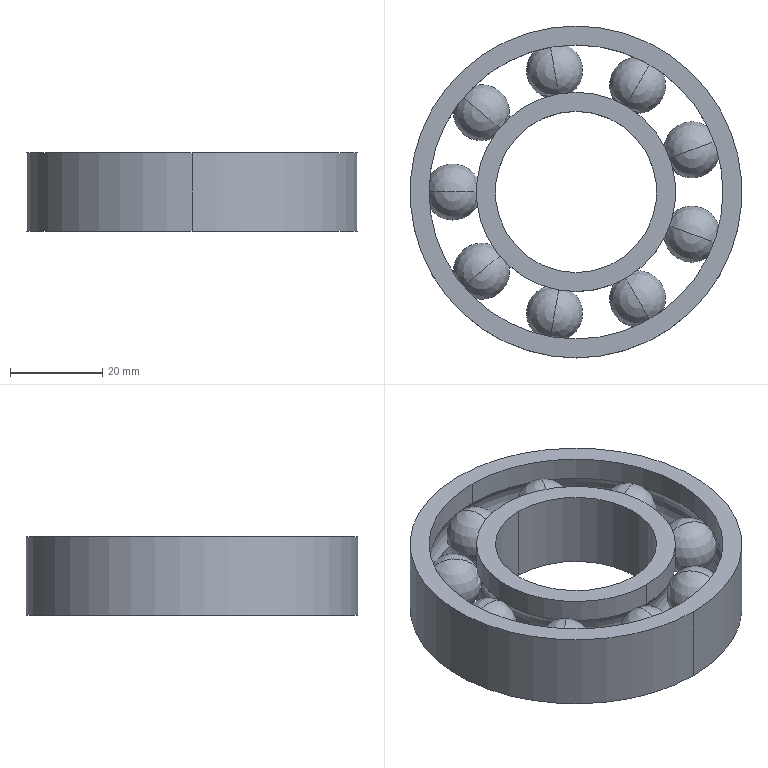Part | NX | features BREP 11 | 11 solids | 38 faces | box 72 x 72 x 17 mm | volume 30735 mm3 | sphere 18 | cylinder 12 | torus 4 | plane 4 | commonest cylinder face diameters 43.222 x4 63.778 x4 35 x2 72 x2
STEP:
#1=CARTESIAN_POINT('',(0.,21.611,3.409));
#2=VERTEX_POINT('',#1);
#3=CARTESIAN_POINT('',(0.,-21.611,3.409));
#4=VERTEX_POINT('',#3);
#5=CARTESIAN_POINT('',(0.,0.,3.409));
#6=DIRECTION('',(0.,0.,1.));
#7=DIRECTION('',(0.,1.,0.));
#8=AXIS2_PLACEMENT_3D('',#5,#6,#7);
#9=CIRCLE('',#8,21.611);
#10=EDGE_CURVE('',#2,#4,#9,.T.);
#11=ORIENTED_EDGE('',*,*,#10,.T.);
#12=CARTESIAN_POINT('',(0.,-21.611,8.5));
#13=VERTEX_POINT('',#12);
#14=CARTESIAN_POINT('',(0.,-21.611,3.409));
#15=DIRECTION('',(0.,0.,1.));
#16=VECTOR('',#15,1000.);
#17=LINE('',#14,#16);
#18=EDGE_CURVE('',#4,#13,#17,.T.);
#19=ORIENTED_EDGE('',*,*,#18,.T.);
#20=CARTESIAN_POINT('',(0.,21.611,8.5));
#21=VERTEX_POINT('',#20);
#22=CARTESIAN_POINT('',(0.,0.,8.5));
#23=DIRECTION('',(0.,0.,1.));
#24=DIRECTION('',(0.,1.,0.));
#25=AXIS2_PLACEMENT_3D('',#22,#23,#24);
#26=CIRCLE('',#25,21.611);
#27=EDGE_CURVE('',#21,#13,#26,.T.);
#28=ORIENTED_EDGE('',*,*,#27,.F.);
#29=CARTESIAN_POINT('',(0.,21.611,3.409));
#30=DIRECTION('',(0.,0.,1.));
#31=VECTOR('',#30,1000.);
#32=LINE('',#29,#31);
#33=EDGE_CURVE('',#2,#21,#32,.T.);
#34=ORIENTED_EDGE('',*,*,#33,.F.);
#35=EDGE_LOOP('',(#11,#19,#28,#34));
#36=FACE_BOUND('',#35,.T.);
#37=CARTESIAN_POINT('',(0.,0.,9.35));
#38=DIRECTION('',(0.,0.,-1.));
#39=DIRECTION('',(0.,1.,0.));
#40=AXIS2_PLACEMENT_3D('',#37,#38,#39);
#41=CYLINDRICAL_SURFACE('',#40,21.611);
#42=ADVANCED_FACE('',(#36),#41,.T.);
#43=CARTESIAN_POINT('',(0.,0.,8.5));
#44=DIRECTION('',(0.,0.,-1.));
#45=DIRECTION('',(0.,1.,0.));
#46=AXIS2_PLACEMENT_3D('',#43,#44,#45);
#47=CIRCLE('',#46,21.611);
#48=EDGE_CURVE('',#21,#13,#47,.T.);
#49=ORIENTED_EDGE('',*,*,#48,.T.);
#50=ORIENTED_EDGE('',*,*,#18,.F.);
#51=CARTESIAN_POINT('',(0.,0.,3.409));
#52=DIRECTION('',(0.,0.,-1.));
#53=DIRECTION('',(0.,1.,0.));
#54=AXIS2_PLACEMENT_3D('',#51,#52,#53);
#55=CIRCLE('',#54,21.611);
#56=EDGE_CURVE('',#2,#4,#55,.T.);
#57=ORIENTED_EDGE('',*,*,#56,.F.);
#58=ORIENTED_EDGE('',*,*,#33,.T.);
#59=EDGE_LOOP('',(#49,#50,#57,#58));
#60=FACE_BOUND('',#59,.T.);
#61=CARTESIAN_POINT('',(0.,0.,9.35));
#62=DIRECTION('',(0.,0.,-1.));
#63=DIRECTION('',(0.,1.,0.));
#64=AXIS2_PLACEMENT_3D('',#61,#62,#63);
#65=CYLINDRICAL_SURFACE('',#64,21.611);
#66=ADVANCED_FACE('',(#60),#65,.T.);
#67=ORIENTED_EDGE('',*,*,#56,.T.);
#68=CARTESIAN_POINT('',(0.,-21.611,-3.409));
#69=VERTEX_POINT('',#68);
#70=CARTESIAN_POINT('',(0.,-26.75,0.));
#71=DIRECTION('',(1.,0.,0.));
#72=DIRECTION('',(0.,0.8333,-0.5528));
#73=AXIS2_PLACEMENT_3D('',#70,#71,#72);
#74=CIRCLE('',#73,6.167);
#75=EDGE_CURVE('',#4,#69,#74,.F.);
#76=ORIENTED_EDGE('',*,*,#75,.T.);
#77=CARTESIAN_POINT('',(0.,21.611,-3.409));
#78=VERTEX_POINT('',#77);
#79=CARTESIAN_POINT('',(0.,0.,-3.409));
#80=DIRECTION('',(0.,0.,-1.));
#81=DIRECTION('',(0.,1.,0.));
#82=AXIS2_PLACEMENT_3D('',#79,#80,#81);
#83=CIRCLE('',#82,21.611);
#84=EDGE_CURVE('',#78,#69,#83,.T.);
#85=ORIENTED_EDGE('',*,*,#84,.F.);
#86=CARTESIAN_POINT('',(0.,26.75,0.));
#87=DIRECTION('',(-1.,0.,0.));
#88=DIRECTION('',(0.,-0.8333,-0.5528));
#89=AXIS2_PLACEMENT_3D('',#86,#87,#88);
#90=CIRCLE('',#89,6.167);
#91=EDGE_CURVE('',#2,#78,#90,.F.);
#92=ORIENTED_EDGE('',*,*,#91,.F.);
#93=EDGE_LOOP('',(#67,#76,#85,#92));
#94=FACE_BOUND('',#93,.T.);
#95=CARTESIAN_POINT('',(0.,0.,0.));
#96=DIRECTION('',(0.,0.,-1.));
#97=DIRECTION('',(0.,1.,0.));
#98=AXIS2_PLACEMENT_3D('',#95,#96,#97);
#99=TOROIDAL_SURFACE('',#98,26.75,6.167);
#100=ADVANCED_FACE('',(#94),#99,.F.);
#101=CARTESIAN_POINT('',(0.,0.,-3.409));
#102=DIRECTION('',(0.,0.,1.));
#103=DIRECTION('',(0.,1.,0.));
#104=AXIS2_PLACEMENT_3D('',#101,#102,#103);
#105=CIRCLE('',#104,21.611);
#106=EDGE_CURVE('',#78,#69,#105,.T.);
#107=ORIENTED_EDGE('',*,*,#106,.T.);
#108=ORIENTED_EDGE('',*,*,#75,.F.);
#109=ORIENTED_EDGE('',*,*,#10,.F.);
#110=ORIENTED_EDGE('',*,*,#91,.T.);
#111=EDGE_LOOP('',(#107,#108,#109,#110));
#112=FACE_BOUND('',#111,.T.);
#113=CARTESIAN_POINT('',(0.,0.,0.));
#114=DIRECTION('',(0.,0.,-1.));
#115=DIRECTION('',(0.,1.,0.));
#116=AXIS2_PLACEMENT_3D('',#113,#114,#115);
#117=TOROIDAL_SURFACE('',#116,26.75,6.167);
#118=ADVANCED_FACE('',(#112),#117,.F.);
#119=CARTESIAN_POINT('',(0.,21.611,-8.5));
#120=VERTEX_POINT('',#119);
#121=CARTESIAN_POINT('',(0.,-21.611,-8.5));
#122=VERTEX_POINT('',#121);
#123=CARTESIAN_POINT('',(0.,0.,-8.5));
#124=DIRECTION('',(0.,0.,1.));
#125=DIRECTION('',(0.,1.,0.));
#126=AXIS2_PLACEMENT_3D('',#123,#124,#125);
#127=CIRCLE('',#126,21.611);
#128=EDGE_CURVE('',#120,#122,#127,.T.);
#129=ORIENTED_EDGE('',*,*,#128,.T.);
#130=CARTESIAN_POINT('',(0.,-21.611,-8.5));
#131=DIRECTION('',(0.,0.,1.));
#132=VECTOR('',#131,1000.);
#133=LINE('',#130,#132);
#134=EDGE_CURVE('',#122,#69,#133,.T.);
#135=ORIENTED_EDGE('',*,*,#134,.T.);
#136=ORIENTED_EDGE('',*,*,#106,.F.);
#137=CARTESIAN_POINT('',(0.,21.611,-8.5));
#138=DIRECTION('',(0.,0.,1.));
#139=VECTOR('',#138,1000.);
#140=LINE('',#137,#139);
#141=EDGE_CURVE('',#120,#78,#140,.T.);
#142=ORIENTED_EDGE('',*,*,#141,.F.);
#143=EDGE_LOOP('',(#129,#135,#136,#142));
#144=FACE_BOUND('',#143,.T.);
#145=CARTESIAN_POINT('',(0.,0.,9.35));
#146=DIRECTION('',(0.,0.,-1.));
#147=DIRECTION('',(0.,1.,0.));
#148=AXIS2_PLACEMENT_3D('',#145,#146,#147);
#149=CYLINDRICAL_SURFACE('',#148,21.611);
#150=ADVANCED_FACE('',(#144),#149,.T.);
#151=ORIENTED_EDGE('',*,*,#84,.T.);
#152=ORIENTED_EDGE('',*,*,#134,.F.);
#153=CARTESIAN_POINT('',(0.,0.,-8.5));
#154=DIRECTION('',(0.,0.,-1.));
#155=DIRECTION('',(0.,1.,0.));
#156=AXIS2_PLACEMENT_3D('',#153,#154,#155);
#157=CIRCLE('',#156,21.611);
#158=EDGE_CURVE('',#120,#122,#157,.T.);
#159=ORIENTED_EDGE('',*,*,#158,.F.);
#160=ORIENTED_EDGE('',*,*,#141,.T.);
#161=EDGE_LOOP('',(#151,#152,#159,#160));
#162=FACE_BOUND('',#161,.T.);
#163=CARTESIAN_POINT('',(0.,0.,9.35));
#164=DIRECTION('',(0.,0.,-1.));
#165=DIRECTION('',(0.,1.,0.));
#166=AXIS2_PLACEMENT_3D('',#163,#164,#165);
#167=CYLINDRICAL_SURFACE('',#166,21.611);
#168=ADVANCED_FACE('',(#162),#167,.T.);
#169=ORIENTED_EDGE('',*,*,#128,.F.);
#170=ORIENTED_EDGE('',*,*,#158,.T.);
#171=EDGE_LOOP('',(#169,#170));
#172=FACE_BOUND('',#171,.T.);
#173=CARTESIAN_POINT('',(0.,17.5,-8.5));
#174=VERTEX_POINT('',#173);
#175=CARTESIAN_POINT('',(0.,-17.5,-8.5));
#176=VERTEX_POINT('',#175);
#177=CARTESIAN_POINT('',(0.,0.,-8.5));
#178=DIRECTION('',(0.,0.,-1.));
#179=DIRECTION('',(0.,1.,0.));
#180=AXIS2_PLACEMENT_3D('',#177,#178,#179);
#181=CIRCLE('',#180,17.5);
#182=EDGE_CURVE('',#174,#176,#181,.T.);
#183=ORIENTED_EDGE('',*,*,#182,.F.);
#184=CARTESIAN_POINT('',(0.,0.,-8.5));
#185=DIRECTION('',(0.,0.,1.));
#186=DIRECTION('',(0.,1.,0.));
#187=AXIS2_PLACEMENT_3D('',#184,#185,#186);
#188=CIRCLE('',#187,17.5);
#189=EDGE_CURVE('',#174,#176,#188,.T.);
#190=ORIENTED_EDGE('',*,*,#189,.T.);
#191=EDGE_LOOP('',(#183,#190));
#192=FACE_BOUND('',#191,.T.);
#193=CARTESIAN_POINT('',(0.,0.,-8.5));
#194=DIRECTION('',(0.,0.,-1.));
#195=DIRECTION('',(0.,1.,0.));
#196=AXIS2_PLACEMENT_3D('',#193,#194,#195);
#197=PLANE('',#196);
#198=ADVANCED_FACE('',(#172,#192),#197,.T.);
#199=CARTESIAN_POINT('',(0.,17.5,8.5));
#200=VERTEX_POINT('',#199);
#201=CARTESIAN_POINT('',(0.,-17.5,8.5));
#202=VERTEX_POINT('',#201);
#203=CARTESIAN_POINT('',(0.,0.,8.5));
#204=DIRECTION('',(0.,0.,1.));
#205=DIRECTION('',(0.,1.,0.));
#206=AXIS2_PLACEMENT_3D('',#203,#204,#205);
#207=CIRCLE('',#206,17.5);
#208=EDGE_CURVE('',#200,#202,#207,.T.);
#209=ORIENTED_EDGE('',*,*,#208,.T.);
#210=CARTESIAN_POINT('',(0.,-17.5,8.5));
#211=DIRECTION('',(0.,0.,-1.));
#212=VECTOR('',#211,1000.);
#213=LINE('',#210,#212);
#214=EDGE_CURVE('',#202,#176,#213,.T.);
#215=ORIENTED_EDGE('',*,*,#214,.T.);
#216=ORIENTED_EDGE('',*,*,#189,.F.);
#217=CARTESIAN_POINT('',(0.,17.5,8.5));
#218=DIRECTION('',(0.,0.,-1.));
#219=VECTOR('',#218,1000.);
#220=LINE('',#217,#219);
#221=EDGE_CURVE('',#200,#174,#220,.T.);
#222=ORIENTED_EDGE('',*,*,#221,.F.);
#223=EDGE_LOOP('',(#209,#215,#216,#222));
#224=FACE_BOUND('',#223,.T.);
#225=CARTESIAN_POINT('',(0.,0.,9.35));
#226=DIRECTION('',(0.,0.,-1.));
#227=DIRECTION('',(0.,1.,0.));
#228=AXIS2_PLACEMENT_3D('',#225,#226,#227);
#229=CYLINDRICAL_SURFACE('',#228,17.5);
#230=ADVANCED_FACE('',(#224),#229,.F.);
#231=ORIENTED_EDGE('',*,*,#182,.T.);
#232=ORIENTED_EDGE('',*,*,#214,.F.);
#233=CARTESIAN_POINT('',(0.,0.,8.5));
#234=DIRECTION('',(0.,0.,-1.));
#235=DIRECTION('',(0.,1.,0.));
#236=AXIS2_PLACEMENT_3D('',#233,#234,#235);
#237=CIRCLE('',#236,17.5);
#238=EDGE_CURVE('',#200,#202,#237,.T.);
#239=ORIENTED_EDGE('',*,*,#238,.F.);
#240=ORIENTED_EDGE('',*,*,#221,.T.);
#241=EDGE_LOOP('',(#231,#232,#239,#240));
#242=FACE_BOUND('',#241,.T.);
#243=CARTESIAN_POINT('',(0.,0.,9.35));
#244=DIRECTION('',(0.,0.,-1.));
#245=DIRECTION('',(0.,1.,0.));
#246=AXIS2_PLACEMENT_3D('',#243,#244,#245);
#247=CYLINDRICAL_SURFACE('',#246,17.5);
#248=ADVANCED_FACE('',(#242),#247,.F.);
#249=ORIENTED_EDGE('',*,*,#48,.F.);
#250=ORIENTED_EDGE('',*,*,#27,.T.);
#251=EDGE_LOOP('',(#249,#250));
#252=FACE_BOUND('',#251,.T.);
#253=ORIENTED_EDGE('',*,*,#208,.F.);
#254=ORIENTED_EDGE('',*,*,#238,.T.);
#255=EDGE_LOOP('',(#253,#254));
#256=FACE_BOUND('',#255,.T.);
#257=CARTESIAN_POINT('',(0.,0.,8.5));
#258=DIRECTION('',(0.,0.,-1.));
#259=DIRECTION('',(0.,1.,0.));
#260=AXIS2_PLACEMENT_3D('',#257,#258,#259);
#261=PLANE('',#260);
#262=ADVANCED_FACE('',(#252,#256),#261,.F.);
#263=CLOSED_SHELL('',(#42,#66,#100,#118,#150,#168,#198,#230,#248,#262));
#264=MANIFOLD_SOLID_BREP('',#263);
#265=CARTESIAN_POINT('',(0.,36.,-8.5));
#266=VERTEX_POINT('',#265);
#267=CARTESIAN_POINT('',(0.,-36.,-8.5));
#268=VERTEX_POINT('',#267);
#269=CARTESIAN_POINT('',(0.,0.,-8.5));
#270=DIRECTION('',(0.,0.,1.));
#271=DIRECTION('',(0.,1.,0.));
#272=AXIS2_PLACEMENT_3D('',#269,#270,#271);
#273=CIRCLE('',#272,36.);
#274=EDGE_CURVE('',#266,#268,#273,.T.);
#275=ORIENTED_EDGE('',*,*,#274,.T.);
#276=CARTESIAN_POINT('',(0.,-36.,8.5));
#277=VERTEX_POINT('',#276);
#278=CARTESIAN_POINT('',(0.,-36.,-8.5));
#279=DIRECTION('',(0.,0.,1.));
#280=VECTOR('',#279,1000.);
#281=LINE('',#278,#280);
#282=EDGE_CURVE('',#268,#277,#281,.T.);
#283=ORIENTED_EDGE('',*,*,#282,.T.);
#284=CARTESIAN_POINT('',(0.,36.,8.5));
#285=VERTEX_POINT('',#284);
#286=CARTESIAN_POINT('',(0.,0.,8.5));
#287=DIRECTION('',(0.,0.,1.));
#288=DIRECTION('',(0.,1.,0.));
#289=AXIS2_PLACEMENT_3D('',#286,#287,#288);
#290=CIRCLE('',#289,36.);
#291=EDGE_CURVE('',#285,#277,#290,.T.);
#292=ORIENTED_EDGE('',*,*,#291,.F.);
#293=CARTESIAN_POINT('',(0.,36.,-8.5));
#294=DIRECTION('',(0.,0.,1.));
#295=VECTOR('',#294,1000.);
#296=LINE('',#293,#295);
#297=EDGE_CURVE('',#266,#285,#296,.T.);
#298=ORIENTED_EDGE('',*,*,#297,.F.);
#299=EDGE_LOOP('',(#275,#283,#292,#298));
#300=FACE_BOUND('',#299,.T.);
#301=CARTESIAN_POINT('',(0.,0.,9.35));
#302=DIRECTION('',(0.,0.,-1.));
#303=DIRECTION('',(0.,1.,0.));
#304=AXIS2_PLACEMENT_3D('',#301,#302,#303);
#305=CYLINDRICAL_SURFACE('',#304,36.);
#306=ADVANCED_FACE('',(#300),#305,.T.);
#307=CARTESIAN_POINT('',(0.,0.,8.5));
#308=DIRECTION('',(0.,0.,-1.));
#309=DIRECTION('',(0.,1.,0.));
#310=AXIS2_PLACEMENT_3D('',#307,#308,#309);
#311=CIRCLE('',#310,36.);
#312=EDGE_CURVE('',#285,#277,#311,.T.);
#313=ORIENTED_EDGE('',*,*,#312,.T.);
#314=ORIENTED_EDGE('',*,*,#282,.F.);
#315=CARTESIAN_POINT('',(0.,0.,-8.5));
#316=DIRECTION('',(0.,0.,-1.));
#317=DIRECTION('',(0.,1.,0.));
#318=AXIS2_PLACEMENT_3D('',#315,#316,#317);
#319=CIRCLE('',#318,36.);
#320=EDGE_CURVE('',#266,#268,#319,.T.);
#321=ORIENTED_EDGE('',*,*,#320,.F.);
#322=ORIENTED_EDGE('',*,*,#297,.T.);
#323=EDGE_LOOP('',(#313,#314,#321,#322));
#324=FACE_BOUND('',#323,.T.);
#325=CARTESIAN_POINT('',(0.,0.,9.35));
#326=DIRECTION('',(0.,0.,-1.));
#327=DIRECTION('',(0.,1.,0.));
#328=AXIS2_PLACEMENT_3D('',#325,#326,#327);
#329=CYLINDRICAL_SURFACE('',#328,36.);
#330=ADVANCED_FACE('',(#324),#329,.T.);
#331=ORIENTED_EDGE('',*,*,#274,.F.);
#332=ORIENTED_EDGE('',*,*,#320,.T.);
#333=EDGE_LOOP('',(#331,#332));
#334=FACE_BOUND('',#333,.T.);
#335=CARTESIAN_POINT('',(0.,31.889,-8.5));
#336=VERTEX_POINT('',#335);
#337=CARTESIAN_POINT('',(0.,-31.889,-8.5));
#338=VERTEX_POINT('',#337);
#339=CARTESIAN_POINT('',(0.,0.,-8.5));
#340=DIRECTION('',(0.,0.,-1.));
#341=DIRECTION('',(0.,1.,0.));
#342=AXIS2_PLACEMENT_3D('',#339,#340,#341);
#343=CIRCLE('',#342,31.889);
#344=EDGE_CURVE('',#336,#338,#343,.T.);
#345=ORIENTED_EDGE('',*,*,#344,.F.);
#346=CARTESIAN_POINT('',(0.,0.,-8.5));
#347=DIRECTION('',(0.,0.,1.));
#348=DIRECTION('',(0.,1.,0.));
#349=AXIS2_PLACEMENT_3D('',#346,#347,#348);
#350=CIRCLE('',#349,31.889);
#351=EDGE_CURVE('',#336,#338,#350,.T.);
#352=ORIENTED_EDGE('',*,*,#351,.T.);
#353=EDGE_LOOP('',(#345,#352));
#354=FACE_BOUND('',#353,.T.);
#355=CARTESIAN_POINT('',(0.,0.,-8.5));
#356=DIRECTION('',(0.,0.,-1.));
#357=DIRECTION('',(0.,1.,0.));
#358=AXIS2_PLACEMENT_3D('',#355,#356,#357);
#359=PLANE('',#358);
#360=ADVANCED_FACE('',(#334,#354),#359,.T.);
#361=CARTESIAN_POINT('',(0.,31.889,-3.409));
#362=VERTEX_POINT('',#361);
#363=CARTESIAN_POINT('',(0.,-31.889,-3.409));
#364=VERTEX_POINT('',#363);
#365=CARTESIAN_POINT('',(0.,0.,-3.409));
#366=DIRECTION('',(0.,0.,1.));
#367=DIRECTION('',(0.,1.,0.));
#368=AXIS2_PLACEMENT_3D('',#365,#366,#367);
#369=CIRCLE('',#368,31.889);
#370=EDGE_CURVE('',#362,#364,#369,.T.);
#371=ORIENTED_EDGE('',*,*,#370,.T.);
#372=CARTESIAN_POINT('',(0.,-31.889,-3.409));
#373=DIRECTION('',(0.,0.,-1.));
#374=VECTOR('',#373,1000.);
#375=LINE('',#372,#374);
#376=EDGE_CURVE('',#364,#338,#375,.T.);
#377=ORIENTED_EDGE('',*,*,#376,.T.);
#378=ORIENTED_EDGE('',*,*,#351,.F.);
#379=CARTESIAN_POINT('',(0.,31.889,-3.409));
#380=DIRECTION('',(0.,0.,-1.));
#381=VECTOR('',#380,1000.);
#382=LINE('',#379,#381);
#383=EDGE_CURVE('',#362,#336,#382,.T.);
#384=ORIENTED_EDGE('',*,*,#383,.F.);
#385=EDGE_LOOP('',(#371,#377,#378,#384));
#386=FACE_BOUND('',#385,.T.);
#387=CARTESIAN_POINT('',(0.,0.,9.35));
#388=DIRECTION('',(0.,0.,-1.));
#389=DIRECTION('',(0.,1.,0.));
#390=AXIS2_PLACEMENT_3D('',#387,#388,#389);
#391=CYLINDRICAL_SURFACE('',#390,31.889);
#392=ADVANCED_FACE('',(#386),#391,.F.);
#393=ORIENTED_EDGE('',*,*,#344,.T.);
#394=ORIENTED_EDGE('',*,*,#376,.F.);
#395=CARTESIAN_POINT('',(0.,0.,-3.409));
#396=DIRECTION('',(0.,0.,-1.));
#397=DIRECTION('',(0.,1.,0.));
#398=AXIS2_PLACEMENT_3D('',#395,#396,#397);
#399=CIRCLE('',#398,31.889);
#400=EDGE_CURVE('',#362,#364,#399,.T.);
#401=ORIENTED_EDGE('',*,*,#400,.F.);
#402=ORIENTED_EDGE('',*,*,#383,.T.);
#403=EDGE_LOOP('',(#393,#394,#401,#402));
#404=FACE_BOUND('',#403,.T.);
#405=CARTESIAN_POINT('',(0.,0.,9.35));
#406=DIRECTION('',(0.,0.,-1.));
#407=DIRECTION('',(0.,1.,0.));
#408=AXIS2_PLACEMENT_3D('',#405,#406,#407);
#409=CYLINDRICAL_SURFACE('',#408,31.889);
#410=ADVANCED_FACE('',(#404),#409,.F.);
#411=ORIENTED_EDGE('',*,*,#400,.T.);
#412=CARTESIAN_POINT('',(0.,-31.889,3.409));
#413=VERTEX_POINT('',#412);
#414=CARTESIAN_POINT('',(0.,-26.75,0.));
#415=DIRECTION('',(1.,0.,0.));
#416=DIRECTION('',(0.,-0.8333,0.5528));
#417=AXIS2_PLACEMENT_3D('',#414,#415,#416);
#418=CIRCLE('',#417,6.167);
#419=EDGE_CURVE('',#364,#413,#418,.F.);
#420=ORIENTED_EDGE('',*,*,#419,.T.);
#421=CARTESIAN_POINT('',(0.,31.889,3.409));
#422=VERTEX_POINT('',#421);
#423=CARTESIAN_POINT('',(0.,0.,3.409));
#424=DIRECTION('',(0.,0.,-1.));
#425=DIRECTION('',(0.,1.,0.));
#426=AXIS2_PLACEMENT_3D('',#423,#424,#425);
#427=CIRCLE('',#426,31.889);
#428=EDGE_CURVE('',#422,#413,#427,.T.);
#429=ORIENTED_EDGE('',*,*,#428,.F.);
#430=CARTESIAN_POINT('',(0.,26.75,0.));
#431=DIRECTION('',(-1.,0.,0.));
#432=DIRECTION('',(0.,0.8333,0.5528));
#433=AXIS2_PLACEMENT_3D('',#430,#431,#432);
#434=CIRCLE('',#433,6.167);
#435=EDGE_CURVE('',#362,#422,#434,.F.);
#436=ORIENTED_EDGE('',*,*,#435,.F.);
#437=EDGE_LOOP('',(#411,#420,#429,#436));
#438=FACE_BOUND('',#437,.T.);
#439=CARTESIAN_POINT('',(0.,0.,0.));
#440=DIRECTION('',(0.,0.,-1.));
#441=DIRECTION('',(0.,1.,0.));
#442=AXIS2_PLACEMENT_3D('',#439,#440,#441);
#443=TOROIDAL_SURFACE('',#442,26.75,6.167);
#444=ADVANCED_FACE('',(#438),#443,.F.);
#445=CARTESIAN_POINT('',(0.,0.,3.409));
#446=DIRECTION('',(0.,0.,1.));
#447=DIRECTION('',(0.,1.,0.));
#448=AXIS2_PLACEMENT_3D('',#445,#446,#447);
#449=CIRCLE('',#448,31.889);
#450=EDGE_CURVE('',#422,#413,#449,.T.);
#451=ORIENTED_EDGE('',*,*,#450,.T.);
#452=ORIENTED_EDGE('',*,*,#419,.F.);
#453=ORIENTED_EDGE('',*,*,#370,.F.);
#454=ORIENTED_EDGE('',*,*,#435,.T.);
#455=EDGE_LOOP('',(#451,#452,#453,#454));
#456=FACE_BOUND('',#455,.T.);
#457=CARTESIAN_POINT('',(0.,0.,0.));
#458=DIRECTION('',(0.,0.,-1.));
#459=DIRECTION('',(0.,1.,0.));
#460=AXIS2_PLACEMENT_3D('',#457,#458,#459);
#461=TOROIDAL_SURFACE('',#460,26.75,6.167);
#462=ADVANCED_FACE('',(#456),#461,.F.);
#463=CARTESIAN_POINT('',(0.,31.889,8.5));
#464=VERTEX_POINT('',#463);
#465=CARTESIAN_POINT('',(0.,-31.889,8.5));
#466=VERTEX_POINT('',#465);
#467=CARTESIAN_POINT('',(0.,0.,8.5));
#468=DIRECTION('',(0.,0.,1.));
#469=DIRECTION('',(0.,1.,0.));
#470=AXIS2_PLACEMENT_3D('',#467,#468,#469);
#471=CIRCLE('',#470,31.889);
#472=EDGE_CURVE('',#464,#466,#471,.T.);
#473=ORIENTED_EDGE('',*,*,#472,.T.);
#474=CARTESIAN_POINT('',(0.,-31.889,8.5));
#475=DIRECTION('',(0.,0.,-1.));
#476=VECTOR('',#475,1000.);
#477=LINE('',#474,#476);
#478=EDGE_CURVE('',#466,#413,#477,.T.);
#479=ORIENTED_EDGE('',*,*,#478,.T.);
#480=ORIENTED_EDGE('',*,*,#450,.F.);
#481=CARTESIAN_POINT('',(0.,31.889,8.5));
#482=DIRECTION('',(0.,0.,-1.));
#483=VECTOR('',#482,1000.);
#484=LINE('',#481,#483);
#485=EDGE_CURVE('',#464,#422,#484,.T.);
#486=ORIENTED_EDGE('',*,*,#485,.F.);
#487=EDGE_LOOP('',(#473,#479,#480,#486));
#488=FACE_BOUND('',#487,.T.);
#489=CARTESIAN_POINT('',(0.,0.,9.35));
#490=DIRECTION('',(0.,0.,-1.));
#491=DIRECTION('',(0.,1.,0.));
#492=AXIS2_PLACEMENT_3D('',#489,#490,#491);
#493=CYLINDRICAL_SURFACE('',#492,31.889);
#494=ADVANCED_FACE('',(#488),#493,.F.);
#495=ORIENTED_EDGE('',*,*,#428,.T.);
#496=ORIENTED_EDGE('',*,*,#478,.F.);
#497=CARTESIAN_POINT('',(0.,0.,8.5));
#498=DIRECTION('',(0.,0.,-1.));
#499=DIRECTION('',(0.,1.,0.));
#500=AXIS2_PLACEMENT_3D('',#497,#498,#499);
#501=CIRCLE('',#500,31.889);
#502=EDGE_CURVE('',#464,#466,#501,.T.);
#503=ORIENTED_EDGE('',*,*,#502,.F.);
#504=ORIENTED_EDGE('',*,*,#485,.T.);
#505=EDGE_LOOP('',(#495,#496,#503,#504));
#506=FACE_BOUND('',#505,.T.);
#507=CARTESIAN_POINT('',(0.,0.,9.35));
#508=DIRECTION('',(0.,0.,-1.));
#509=DIRECTION('',(0.,1.,0.));
#510=AXIS2_PLACEMENT_3D('',#507,#508,#509);
#511=CYLINDRICAL_SURFACE('',#510,31.889);
#512=ADVANCED_FACE('',(#506),#511,.F.);
#513=ORIENTED_EDGE('',*,*,#312,.F.);
#514=ORIENTED_EDGE('',*,*,#291,.T.);
#515=EDGE_LOOP('',(#513,#514));
#516=FACE_BOUND('',#515,.T.);
#517=ORIENTED_EDGE('',*,*,#472,.F.);
#518=ORIENTED_EDGE('',*,*,#502,.T.);
#519=EDGE_LOOP('',(#517,#518));
#520=FACE_BOUND('',#519,.T.);
#521=CARTESIAN_POINT('',(0.,0.,8.5));
#522=DIRECTION('',(0.,0.,-1.));
#523=DIRECTION('',(0.,1.,0.));
#524=AXIS2_PLACEMENT_3D('',#521,#522,#523);
#525=PLANE('',#524);
#526=ADVANCED_FACE('',(#516,#520),#525,.F.);
#527=CLOSED_SHELL('',(#306,#330,#360,#392,#410,#444,#462,#494,#512,#526));
#528=MANIFOLD_SOLID_BREP('',#527);
#529=CARTESIAN_POINT('',(13.375,23.166,6.167));
#530=VERTEX_POINT('',#529);
#531=CARTESIAN_POINT('',(13.375,23.166,-6.167));
#532=VERTEX_POINT('',#531);
#533=CARTESIAN_POINT('',(13.375,23.166,0.));
#534=DIRECTION('',(-0.866,0.5,0.));
#535=DIRECTION('',(0.,0.,-1.));
#536=AXIS2_PLACEMENT_3D('',#533,#534,#535);
#537=CIRCLE('',#536,6.167);
#538=EDGE_CURVE('',#530,#532,#537,.F.);
#539=ORIENTED_EDGE('',*,*,#538,.T.);
#540=CARTESIAN_POINT('',(13.375,23.166,0.));
#541=DIRECTION('',(0.866,-0.5,0.));
#542=DIRECTION('',(0.,0.,-1.));
#543=AXIS2_PLACEMENT_3D('',#540,#541,#542);
#544=CIRCLE('',#543,6.167);
#545=EDGE_CURVE('',#530,#532,#544,.F.);
#546=ORIENTED_EDGE('',*,*,#545,.F.);
#547=EDGE_LOOP('',(#539,#546));
#548=FACE_BOUND('',#547,.T.);
#549=CARTESIAN_POINT('',(13.375,23.166,0.));
#550=DIRECTION('',(0.,0.,-1.));
#551=DIRECTION('',(0.5,0.866,0.));
#552=AXIS2_PLACEMENT_3D('',#549,#550,#551);
#553=SPHERICAL_SURFACE('',#552,6.167);
#554=ADVANCED_FACE('',(#548),#553,.T.);
#555=ORIENTED_EDGE('',*,*,#538,.F.);
#556=ORIENTED_EDGE('',*,*,#545,.T.);
#557=EDGE_LOOP('',(#555,#556));
#558=FACE_BOUND('',#557,.T.);
#559=CARTESIAN_POINT('',(13.375,23.166,0.));
#560=DIRECTION('',(0.,0.,-1.));
#561=DIRECTION('',(0.5,0.866,0.));
#562=AXIS2_PLACEMENT_3D('',#559,#560,#561);
#563=SPHERICAL_SURFACE('',#562,6.167);
#564=ADVANCED_FACE('',(#558),#563,.T.);
#565=CLOSED_SHELL('',(#554,#564));
#566=MANIFOLD_SOLID_BREP('',#565);
#567=CARTESIAN_POINT('',(25.137,9.149,6.167));
#568=VERTEX_POINT('',#567);
#569=CARTESIAN_POINT('',(25.137,9.149,-6.167));
#570=VERTEX_POINT('',#569);
#571=CARTESIAN_POINT('',(25.137,9.149,0.));
#572=DIRECTION('',(-0.342,0.9397,0.));
#573=DIRECTION('',(0.,0.,-1.));
#574=AXIS2_PLACEMENT_3D('',#571,#572,#573);
#575=CIRCLE('',#574,6.167);
#576=EDGE_CURVE('',#568,#570,#575,.F.);
#577=ORIENTED_EDGE('',*,*,#576,.T.);
#578=CARTESIAN_POINT('',(25.137,9.149,0.));
#579=DIRECTION('',(0.342,-0.9397,0.));
#580=DIRECTION('',(0.,0.,-1.));
#581=AXIS2_PLACEMENT_3D('',#578,#579,#580);
#582=CIRCLE('',#581,6.167);
#583=EDGE_CURVE('',#568,#570,#582,.F.);
#584=ORIENTED_EDGE('',*,*,#583,.F.);
#585=EDGE_LOOP('',(#577,#584));
#586=FACE_BOUND('',#585,.T.);
#587=CARTESIAN_POINT('',(25.137,9.149,0.));
#588=DIRECTION('',(0.,0.,-1.));
#589=DIRECTION('',(0.9397,0.342,0.));
#590=AXIS2_PLACEMENT_3D('',#587,#588,#589);
#591=SPHERICAL_SURFACE('',#590,6.167);
#592=ADVANCED_FACE('',(#586),#591,.T.);
#593=ORIENTED_EDGE('',*,*,#576,.F.);
#594=ORIENTED_EDGE('',*,*,#583,.T.);
#595=EDGE_LOOP('',(#593,#594));
#596=FACE_BOUND('',#595,.T.);
#597=CARTESIAN_POINT('',(25.137,9.149,0.));
#598=DIRECTION('',(0.,0.,-1.));
#599=DIRECTION('',(0.9397,0.342,0.));
#600=AXIS2_PLACEMENT_3D('',#597,#598,#599);
#601=SPHERICAL_SURFACE('',#600,6.167);
#602=ADVANCED_FACE('',(#596),#601,.T.);
#603=CLOSED_SHELL('',(#592,#602));
#604=MANIFOLD_SOLID_BREP('',#603);
#605=CARTESIAN_POINT('',(25.137,-9.149,6.167));
#606=VERTEX_POINT('',#605);
#607=CARTESIAN_POINT('',(25.137,-9.149,-6.167));
#608=VERTEX_POINT('',#607);
#609=CARTESIAN_POINT('',(25.137,-9.149,0.));
#610=DIRECTION('',(0.342,0.9397,0.));
#611=DIRECTION('',(0.,0.,-1.));
#612=AXIS2_PLACEMENT_3D('',#609,#610,#611);
#613=CIRCLE('',#612,6.167);
#614=EDGE_CURVE('',#606,#608,#613,.F.);
#615=ORIENTED_EDGE('',*,*,#614,.T.);
#616=CARTESIAN_POINT('',(25.137,-9.149,0.));
#617=DIRECTION('',(-0.342,-0.9397,0.));
#618=DIRECTION('',(0.,0.,-1.));
#619=AXIS2_PLACEMENT_3D('',#616,#617,#618);
#620=CIRCLE('',#619,6.167);
#621=EDGE_CURVE('',#606,#608,#620,.F.);
#622=ORIENTED_EDGE('',*,*,#621,.F.);
#623=EDGE_LOOP('',(#615,#622));
#624=FACE_BOUND('',#623,.T.);
#625=CARTESIAN_POINT('',(25.137,-9.149,0.));
#626=DIRECTION('',(0.,0.,-1.));
#627=DIRECTION('',(0.9397,-0.342,0.));
#628=AXIS2_PLACEMENT_3D('',#625,#626,#627);
#629=SPHERICAL_SURFACE('',#628,6.167);
#630=ADVANCED_FACE('',(#624),#629,.T.);
#631=ORIENTED_EDGE('',*,*,#614,.F.);
#632=ORIENTED_EDGE('',*,*,#621,.T.);
#633=EDGE_LOOP('',(#631,#632));
#634=FACE_BOUND('',#633,.T.);
#635=CARTESIAN_POINT('',(25.137,-9.149,0.));
#636=DIRECTION('',(0.,0.,-1.));
#637=DIRECTION('',(0.9397,-0.342,0.));
#638=AXIS2_PLACEMENT_3D('',#635,#636,#637);
#639=SPHERICAL_SURFACE('',#638,6.167);
#640=ADVANCED_FACE('',(#634),#639,.T.);
#641=CLOSED_SHELL('',(#630,#640));
#642=MANIFOLD_SOLID_BREP('',#641);
#643=CARTESIAN_POINT('',(13.375,-23.166,6.167));
#644=VERTEX_POINT('',#643);
#645=CARTESIAN_POINT('',(13.375,-23.166,-6.167));
#646=VERTEX_POINT('',#645);
#647=CARTESIAN_POINT('',(13.375,-23.166,0.));
#648=DIRECTION('',(0.866,0.5,0.));
#649=DIRECTION('',(0.,0.,-1.));
#650=AXIS2_PLACEMENT_3D('',#647,#648,#649);
#651=CIRCLE('',#650,6.167);
#652=EDGE_CURVE('',#644,#646,#651,.F.);
#653=ORIENTED_EDGE('',*,*,#652,.T.);
#654=CARTESIAN_POINT('',(13.375,-23.166,0.));
#655=DIRECTION('',(-0.866,-0.5,0.));
#656=DIRECTION('',(0.,0.,-1.));
#657=AXIS2_PLACEMENT_3D('',#654,#655,#656);
#658=CIRCLE('',#657,6.167);
#659=EDGE_CURVE('',#644,#646,#658,.F.);
#660=ORIENTED_EDGE('',*,*,#659,.F.);
#661=EDGE_LOOP('',(#653,#660));
#662=FACE_BOUND('',#661,.T.);
#663=CARTESIAN_POINT('',(13.375,-23.166,0.));
#664=DIRECTION('',(0.,0.,-1.));
#665=DIRECTION('',(0.5,-0.866,0.));
#666=AXIS2_PLACEMENT_3D('',#663,#664,#665);
#667=SPHERICAL_SURFACE('',#666,6.167);
#668=ADVANCED_FACE('',(#662),#667,.T.);
#669=ORIENTED_EDGE('',*,*,#652,.F.);
#670=ORIENTED_EDGE('',*,*,#659,.T.);
#671=EDGE_LOOP('',(#669,#670));
#672=FACE_BOUND('',#671,.T.);
#673=CARTESIAN_POINT('',(13.375,-23.166,0.));
#674=DIRECTION('',(0.,0.,-1.));
#675=DIRECTION('',(0.5,-0.866,0.));
#676=AXIS2_PLACEMENT_3D('',#673,#674,#675);
#677=SPHERICAL_SURFACE('',#676,6.167);
#678=ADVANCED_FACE('',(#672),#677,.T.);
#679=CLOSED_SHELL('',(#668,#678));
#680=MANIFOLD_SOLID_BREP('',#679);
#681=CARTESIAN_POINT('',(-4.645,-26.344,-6.167));
#682=VERTEX_POINT('',#681);
#683=CARTESIAN_POINT('',(-4.645,-26.344,6.167));
#684=VERTEX_POINT('',#683);
#685=CARTESIAN_POINT('',(-4.645,-26.344,0.));
#686=DIRECTION('',(0.9848,-0.1736,0.));
#687=DIRECTION('',(0.,0.,-1.));
#688=AXIS2_PLACEMENT_3D('',#685,#686,#687);
#689=CIRCLE('',#688,6.167);
#690=EDGE_CURVE('',#682,#684,#689,.T.);
#691=ORIENTED_EDGE('',*,*,#690,.F.);
#692=CARTESIAN_POINT('',(-4.645,-26.344,0.));
#693=DIRECTION('',(-0.9848,0.1736,0.));
#694=DIRECTION('',(0.,0.,-1.));
#695=AXIS2_PLACEMENT_3D('',#692,#693,#694);
#696=CIRCLE('',#695,6.167);
#697=EDGE_CURVE('',#682,#684,#696,.T.);
#698=ORIENTED_EDGE('',*,*,#697,.T.);
#699=EDGE_LOOP('',(#691,#698));
#700=FACE_BOUND('',#699,.T.);
#701=CARTESIAN_POINT('',(-4.645,-26.344,0.));
#702=DIRECTION('',(0.,0.,-1.));
#703=DIRECTION('',(-0.1736,-0.9848,0.));
#704=AXIS2_PLACEMENT_3D('',#701,#702,#703);
#705=SPHERICAL_SURFACE('',#704,6.167);
#706=ADVANCED_FACE('',(#700),#705,.T.);
#707=ORIENTED_EDGE('',*,*,#690,.T.);
#708=ORIENTED_EDGE('',*,*,#697,.F.);
#709=EDGE_LOOP('',(#707,#708));
#710=FACE_BOUND('',#709,.T.);
#711=CARTESIAN_POINT('',(-4.645,-26.344,0.));
#712=DIRECTION('',(0.,0.,-1.));
#713=DIRECTION('',(-0.1736,-0.9848,0.));
#714=AXIS2_PLACEMENT_3D('',#711,#712,#713);
#715=SPHERICAL_SURFACE('',#714,6.167);
#716=ADVANCED_FACE('',(#710),#715,.T.);
#717=CLOSED_SHELL('',(#706,#716));
#718=MANIFOLD_SOLID_BREP('',#717);
#719=CARTESIAN_POINT('',(-20.492,-17.195,-6.167));
#720=VERTEX_POINT('',#719);
#721=CARTESIAN_POINT('',(-20.492,-17.195,6.167));
#722=VERTEX_POINT('',#721);
#723=CARTESIAN_POINT('',(-20.492,-17.195,0.));
#724=DIRECTION('',(0.6428,-0.766,0.));
#725=DIRECTION('',(0.,0.,-1.));
#726=AXIS2_PLACEMENT_3D('',#723,#724,#725);
#727=CIRCLE('',#726,6.167);
#728=EDGE_CURVE('',#720,#722,#727,.T.);
#729=ORIENTED_EDGE('',*,*,#728,.F.);
#730=CARTESIAN_POINT('',(-20.492,-17.195,0.));
#731=DIRECTION('',(-0.6428,0.766,0.));
#732=DIRECTION('',(0.,0.,-1.));
#733=AXIS2_PLACEMENT_3D('',#730,#731,#732);
#734=CIRCLE('',#733,6.167);
#735=EDGE_CURVE('',#720,#722,#734,.T.);
#736=ORIENTED_EDGE('',*,*,#735,.T.);
#737=EDGE_LOOP('',(#729,#736));
#738=FACE_BOUND('',#737,.T.);
#739=CARTESIAN_POINT('',(-20.492,-17.195,0.));
#740=DIRECTION('',(0.,0.,-1.));
#741=DIRECTION('',(-0.766,-0.6428,0.));
#742=AXIS2_PLACEMENT_3D('',#739,#740,#741);
#743=SPHERICAL_SURFACE('',#742,6.167);
#744=ADVANCED_FACE('',(#738),#743,.T.);
#745=ORIENTED_EDGE('',*,*,#728,.T.);
#746=ORIENTED_EDGE('',*,*,#735,.F.);
#747=EDGE_LOOP('',(#745,#746));
#748=FACE_BOUND('',#747,.T.);
#749=CARTESIAN_POINT('',(-20.492,-17.195,0.));
#750=DIRECTION('',(0.,0.,-1.));
#751=DIRECTION('',(-0.766,-0.6428,0.));
#752=AXIS2_PLACEMENT_3D('',#749,#750,#751);
#753=SPHERICAL_SURFACE('',#752,6.167);
#754=ADVANCED_FACE('',(#748),#753,.T.);
#755=CLOSED_SHELL('',(#744,#754));
#756=MANIFOLD_SOLID_BREP('',#755);
#757=CARTESIAN_POINT('',(-26.75,0.,-6.167));
#758=VERTEX_POINT('',#757);
#759=CARTESIAN_POINT('',(-26.75,0.,6.167));
#760=VERTEX_POINT('',#759);
#761=CARTESIAN_POINT('',(-26.75,0.,0.));
#762=DIRECTION('',(0.,-1.,0.));
#763=DIRECTION('',(0.,0.,-1.));
#764=AXIS2_PLACEMENT_3D('',#761,#762,#763);
#765=CIRCLE('',#764,6.167);
#766=EDGE_CURVE('',#758,#760,#765,.T.);
#767=ORIENTED_EDGE('',*,*,#766,.F.);
#768=CARTESIAN_POINT('',(-26.75,0.,0.));
#769=DIRECTION('',(0.,1.,0.));
#770=DIRECTION('',(0.,0.,-1.));
#771=AXIS2_PLACEMENT_3D('',#768,#769,#770);
#772=CIRCLE('',#771,6.167);
#773=EDGE_CURVE('',#758,#760,#772,.T.);
#774=ORIENTED_EDGE('',*,*,#773,.T.);
#775=EDGE_LOOP('',(#767,#774));
#776=FACE_BOUND('',#775,.T.);
#777=CARTESIAN_POINT('',(-26.75,0.,0.));
#778=DIRECTION('',(0.,0.,-1.));
#779=DIRECTION('',(-1.,0.,0.));
#780=AXIS2_PLACEMENT_3D('',#777,#778,#779);
#781=SPHERICAL_SURFACE('',#780,6.167);
#782=ADVANCED_FACE('',(#776),#781,.T.);
#783=ORIENTED_EDGE('',*,*,#766,.T.);
#784=ORIENTED_EDGE('',*,*,#773,.F.);
#785=EDGE_LOOP('',(#783,#784));
#786=FACE_BOUND('',#785,.T.);
#787=CARTESIAN_POINT('',(-26.75,0.,0.));
#788=DIRECTION('',(0.,0.,-1.));
#789=DIRECTION('',(-1.,0.,0.));
#790=AXIS2_PLACEMENT_3D('',#787,#788,#789);
#791=SPHERICAL_SURFACE('',#790,6.167);
#792=ADVANCED_FACE('',(#786),#791,.T.);
#793=CLOSED_SHELL('',(#782,#792));
#794=MANIFOLD_SOLID_BREP('',#793);
#795=CARTESIAN_POINT('',(-20.492,17.195,-6.167));
#796=VERTEX_POINT('',#795);
#797=CARTESIAN_POINT('',(-20.492,17.195,6.167));
#798=VERTEX_POINT('',#797);
#799=CARTESIAN_POINT('',(-20.492,17.195,0.));
#800=DIRECTION('',(-0.6428,-0.766,0.));
#801=DIRECTION('',(0.,0.,-1.));
#802=AXIS2_PLACEMENT_3D('',#799,#800,#801);
#803=CIRCLE('',#802,6.167);
#804=EDGE_CURVE('',#796,#798,#803,.T.);
#805=ORIENTED_EDGE('',*,*,#804,.F.);
#806=CARTESIAN_POINT('',(-20.492,17.195,0.));
#807=DIRECTION('',(0.6428,0.766,0.));
#808=DIRECTION('',(0.,0.,-1.));
#809=AXIS2_PLACEMENT_3D('',#806,#807,#808);
#810=CIRCLE('',#809,6.167);
#811=EDGE_CURVE('',#796,#798,#810,.T.);
#812=ORIENTED_EDGE('',*,*,#811,.T.);
#813=EDGE_LOOP('',(#805,#812));
#814=FACE_BOUND('',#813,.T.);
#815=CARTESIAN_POINT('',(-20.492,17.195,0.));
#816=DIRECTION('',(0.,0.,-1.));
#817=DIRECTION('',(-0.766,0.6428,0.));
#818=AXIS2_PLACEMENT_3D('',#815,#816,#817);
#819=SPHERICAL_SURFACE('',#818,6.167);
#820=ADVANCED_FACE('',(#814),#819,.T.);
#821=ORIENTED_EDGE('',*,*,#804,.T.);
#822=ORIENTED_EDGE('',*,*,#811,.F.);
#823=EDGE_LOOP('',(#821,#822));
#824=FACE_BOUND('',#823,.T.);
#825=CARTESIAN_POINT('',(-20.492,17.195,0.));
#826=DIRECTION('',(0.,0.,-1.));
#827=DIRECTION('',(-0.766,0.6428,0.));
#828=AXIS2_PLACEMENT_3D('',#825,#826,#827);
#829=SPHERICAL_SURFACE('',#828,6.167);
#830=ADVANCED_FACE('',(#824),#829,.T.);
#831=CLOSED_SHELL('',(#820,#830));
#832=MANIFOLD_SOLID_BREP('',#831);
#833=CARTESIAN_POINT('',(-4.645,26.344,-6.167));
#834=VERTEX_POINT('',#833);
#835=CARTESIAN_POINT('',(-4.645,26.344,6.167));
#836=VERTEX_POINT('',#835);
#837=CARTESIAN_POINT('',(-4.645,26.344,0.));
#838=DIRECTION('',(-0.9848,-0.1736,0.));
#839=DIRECTION('',(0.,0.,-1.));
#840=AXIS2_PLACEMENT_3D('',#837,#838,#839);
#841=CIRCLE('',#840,6.167);
#842=EDGE_CURVE('',#834,#836,#841,.T.);
#843=ORIENTED_EDGE('',*,*,#842,.F.);
#844=CARTESIAN_POINT('',(-4.645,26.344,0.));
#845=DIRECTION('',(0.9848,0.1736,0.));
#846=DIRECTION('',(0.,0.,-1.));
#847=AXIS2_PLACEMENT_3D('',#844,#845,#846);
#848=CIRCLE('',#847,6.167);
#849=EDGE_CURVE('',#834,#836,#848,.T.);
#850=ORIENTED_EDGE('',*,*,#849,.T.);
#851=EDGE_LOOP('',(#843,#850));
#852=FACE_BOUND('',#851,.T.);
#853=CARTESIAN_POINT('',(-4.645,26.344,0.));
#854=DIRECTION('',(0.,0.,-1.));
#855=DIRECTION('',(-0.1736,0.9848,0.));
#856=AXIS2_PLACEMENT_3D('',#853,#854,#855);
#857=SPHERICAL_SURFACE('',#856,6.167);
#858=ADVANCED_FACE('',(#852),#857,.T.);
#859=ORIENTED_EDGE('',*,*,#842,.T.);
#860=ORIENTED_EDGE('',*,*,#849,.F.);
#861=EDGE_LOOP('',(#859,#860));
#862=FACE_BOUND('',#861,.T.);
#863=CARTESIAN_POINT('',(-4.645,26.344,0.));
#864=DIRECTION('',(0.,0.,-1.));
#865=DIRECTION('',(-0.1736,0.9848,0.));
#866=AXIS2_PLACEMENT_3D('',#863,#864,#865);
#867=SPHERICAL_SURFACE('',#866,6.167);
#868=ADVANCED_FACE('',(#862),#867,.T.);
#869=CLOSED_SHELL('',(#858,#868));
#870=MANIFOLD_SOLID_BREP('',#869);
#871=(LENGTH_UNIT()NAMED_UNIT(*)SI_UNIT(.MILLI.,.METRE.));
#872=UNCERTAINTY_MEASURE_WITH_UNIT(LENGTH_MEASURE(0.00001),#871,'','');
#873=(NAMED_UNIT(*)PLANE_ANGLE_UNIT()SI_UNIT($,.RADIAN.));
#874=(NAMED_UNIT(*)SI_UNIT($,.STERADIAN.)SOLID_ANGLE_UNIT());
#875=(GEOMETRIC_REPRESENTATION_CONTEXT(3)GLOBAL_UNCERTAINTY_ASSIGNED_CONTEXT((#872))GLOBAL_UNIT_ASSIGNED_CONTEXT((#871,#873,#874))REPRESENTATION_CONTEXT('',''));
#876=ADVANCED_BREP_SHAPE_REPRESENTATION('',(#264,#528,#566,#604,#642,#680,#718,#756,#794,#832,#870),#875);